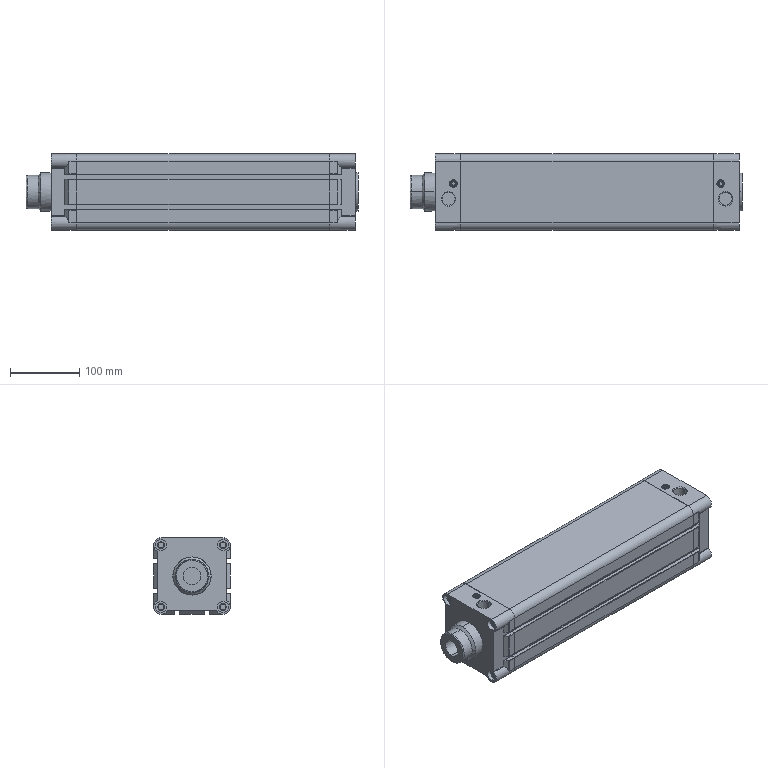Part | STEP file | _SE-100x300-CR (0) | 1 solid | 398 faces | box 478 x 110 x 110 mm | volume 2351296 mm3 | cylinder 190 | plane 176 | cone 30 | spline 2 | commonest cylinder face diameters 1 x90 8.376 x16 15.9 x16 22 x16 2 x12 21 x10